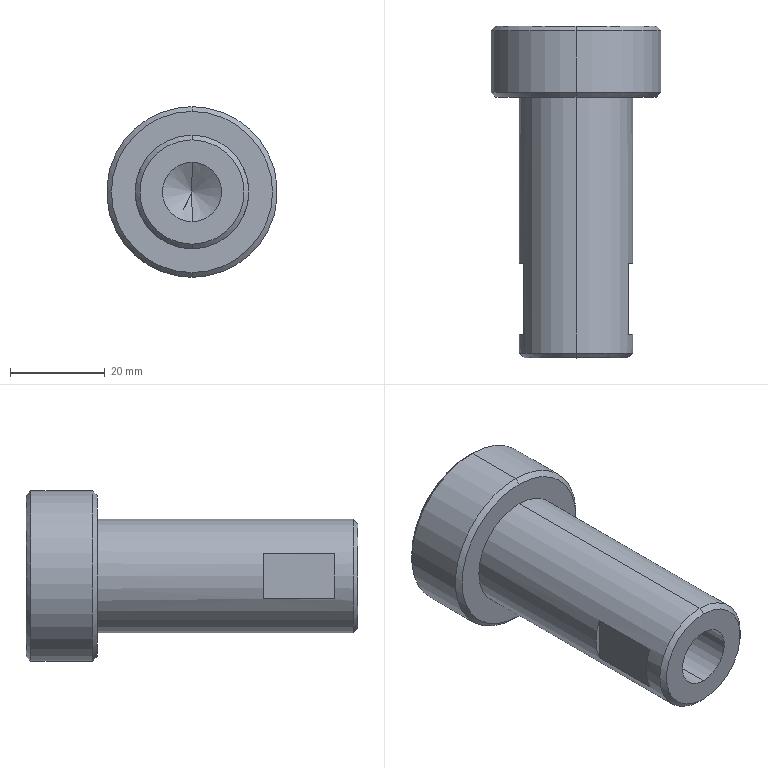Part | SolidWorks | features Chamfer 1, HoleWzd 1, ICE 1, Revolution 1 | 1 solid | 23 faces | box 36 x 70 x 36 mm | volume 37200 mm3 | plane 9 | cone 8 | cylinder 6 | commonest cylinder face diameters 12.5 x2 24 x2 36 x2
STEP:
#1=CARTESIAN_POINT('',(0.,-1.346,6.25));
#2=VERTEX_POINT('',#1);
#3=CARTESIAN_POINT('',(0.,-1.346,-6.25));
#4=VERTEX_POINT('',#3);
#5=CARTESIAN_POINT('',(0.,-1.346,0.));
#6=DIRECTION('',(0.,-1.,0.));
#7=DIRECTION('',(0.,0.,-1.));
#8=AXIS2_PLACEMENT_3D('',#5,#6,#7);
#9=CIRCLE('',#8,6.25);
#10=EDGE_CURVE('',#2,#4,#9,.T.);
#11=ORIENTED_EDGE('',*,*,#10,.F.);
#12=CARTESIAN_POINT('',(0.,-21.346,6.25));
#13=VERTEX_POINT('',#12);
#14=CARTESIAN_POINT('',(0.,-21.346,6.25));
#15=DIRECTION('',(0.,-1.,0.));
#16=VECTOR('',#15,1000.);
#17=LINE('',#14,#16);
#18=EDGE_CURVE('',#2,#13,#17,.T.);
#19=ORIENTED_EDGE('',*,*,#18,.T.);
#20=CARTESIAN_POINT('',(0.,-21.346,-6.25));
#21=VERTEX_POINT('',#20);
#22=CARTESIAN_POINT('',(0.,-21.346,0.));
#23=DIRECTION('',(0.,-1.,0.));
#24=DIRECTION('',(0.,0.,-1.));
#25=AXIS2_PLACEMENT_3D('',#22,#23,#24);
#26=CIRCLE('',#25,6.25);
#27=EDGE_CURVE('',#13,#21,#26,.T.);
#28=ORIENTED_EDGE('',*,*,#27,.T.);
#29=CARTESIAN_POINT('',(0.,-21.346,-6.25));
#30=DIRECTION('',(0.,-1.,0.));
#31=VECTOR('',#30,1000.);
#32=LINE('',#29,#31);
#33=EDGE_CURVE('',#4,#21,#32,.T.);
#34=ORIENTED_EDGE('',*,*,#33,.F.);
#35=EDGE_LOOP('',(#11,#19,#28,#34));
#36=FACE_OUTER_BOUND('',#35,.T.);
#37=CARTESIAN_POINT('',(0.,-21.346,0.));
#38=DIRECTION('',(0.,-1.,0.));
#39=DIRECTION('',(0.,0.,-1.));
#40=AXIS2_PLACEMENT_3D('',#37,#38,#39);
#41=CYLINDRICAL_SURFACE('',#40,6.25);
#42=ADVANCED_FACE('',(#36),#41,.F.);
#43=CARTESIAN_POINT('',(0.,2.409,0.));
#44=VERTEX_POINT('',#43);
#45=CARTESIAN_POINT('',(0.,-1.346,-6.25));
#46=DIRECTION('',(0.,-0.515,-0.8572));
#47=VECTOR('',#46,1000.);
#48=LINE('',#45,#47);
#49=EDGE_CURVE('',#44,#4,#48,.T.);
#50=ORIENTED_EDGE('',*,*,#49,.F.);
#51=CARTESIAN_POINT('',(0.,-1.346,6.25));
#52=DIRECTION('',(0.,-0.515,0.8572));
#53=VECTOR('',#52,1000.);
#54=LINE('',#51,#53);
#55=EDGE_CURVE('',#44,#2,#54,.T.);
#56=ORIENTED_EDGE('',*,*,#55,.T.);
#57=ORIENTED_EDGE('',*,*,#10,.T.);
#58=EDGE_LOOP('',(#50,#56,#57));
#59=FACE_OUTER_BOUND('',#58,.T.);
#60=CARTESIAN_POINT('',(0.,-1.346,0.));
#61=DIRECTION('',(0.,-1.,0.));
#62=DIRECTION('',(0.,0.,-1.));
#63=AXIS2_PLACEMENT_3D('',#60,#61,#62);
#64=CONICAL_SURFACE('',#63,6.25,1.03);
#65=ADVANCED_FACE('',(#59),#64,.F.);
#66=CARTESIAN_POINT('',(0.,48.654,17.));
#67=VERTEX_POINT('',#66);
#68=CARTESIAN_POINT('',(0.,48.654,-17.));
#69=VERTEX_POINT('',#68);
#70=CARTESIAN_POINT('',(0.,48.654,0.));
#71=DIRECTION('',(0.,1.,0.));
#72=DIRECTION('',(0.,0.,1.));
#73=AXIS2_PLACEMENT_3D('',#70,#71,#72);
#74=CIRCLE('',#73,17.);
#75=EDGE_CURVE('',#67,#69,#74,.T.);
#76=ORIENTED_EDGE('',*,*,#75,.F.);
#77=CARTESIAN_POINT('',(0.,47.654,18.));
#78=VERTEX_POINT('',#77);
#79=CARTESIAN_POINT('',(0.,48.654,17.));
#80=DIRECTION('',(0.,-0.7071,0.7071));
#81=VECTOR('',#80,1000.);
#82=LINE('',#79,#81);
#83=EDGE_CURVE('',#67,#78,#82,.T.);
#84=ORIENTED_EDGE('',*,*,#83,.T.);
#85=CARTESIAN_POINT('',(0.,47.654,-18.));
#86=VERTEX_POINT('',#85);
#87=CARTESIAN_POINT('',(0.,47.654,0.));
#88=DIRECTION('',(0.,-1.,0.));
#89=DIRECTION('',(0.,0.,1.));
#90=AXIS2_PLACEMENT_3D('',#87,#88,#89);
#91=CIRCLE('',#90,18.);
#92=EDGE_CURVE('',#86,#78,#91,.T.);
#93=ORIENTED_EDGE('',*,*,#92,.F.);
#94=CARTESIAN_POINT('',(0.,48.654,-17.));
#95=DIRECTION('',(0.,-0.7071,-0.7071));
#96=VECTOR('',#95,1000.);
#97=LINE('',#94,#96);
#98=EDGE_CURVE('',#69,#86,#97,.T.);
#99=ORIENTED_EDGE('',*,*,#98,.F.);
#100=EDGE_LOOP('',(#76,#84,#93,#99));
#101=FACE_OUTER_BOUND('',#100,.T.);
#102=CARTESIAN_POINT('',(0.,48.654,0.));
#103=DIRECTION('',(0.,-1.,0.));
#104=DIRECTION('',(0.,0.,-1.));
#105=AXIS2_PLACEMENT_3D('',#102,#103,#104);
#106=CONICAL_SURFACE('',#105,17.,0.7854);
#107=ADVANCED_FACE('',(#101),#106,.T.);
#108=CARTESIAN_POINT('',(0.,33.654,-17.));
#109=VERTEX_POINT('',#108);
#110=CARTESIAN_POINT('',(0.,33.654,17.));
#111=VERTEX_POINT('',#110);
#112=CARTESIAN_POINT('',(0.,33.654,0.));
#113=DIRECTION('',(0.,-1.,0.));
#114=DIRECTION('',(0.,0.,-1.));
#115=AXIS2_PLACEMENT_3D('',#112,#113,#114);
#116=CIRCLE('',#115,17.);
#117=EDGE_CURVE('',#109,#111,#116,.T.);
#118=ORIENTED_EDGE('',*,*,#117,.F.);
#119=CARTESIAN_POINT('',(0.,34.654,-18.));
#120=VERTEX_POINT('',#119);
#121=CARTESIAN_POINT('',(0.,34.654,-18.));
#122=DIRECTION('',(0.,0.7071,-0.7071));
#123=VECTOR('',#122,1000.);
#124=LINE('',#121,#123);
#125=EDGE_CURVE('',#109,#120,#124,.T.);
#126=ORIENTED_EDGE('',*,*,#125,.T.);
#127=CARTESIAN_POINT('',(0.,34.654,18.));
#128=VERTEX_POINT('',#127);
#129=CARTESIAN_POINT('',(0.,34.654,0.));
#130=DIRECTION('',(0.,1.,0.));
#131=DIRECTION('',(0.,0.,-1.));
#132=AXIS2_PLACEMENT_3D('',#129,#130,#131);
#133=CIRCLE('',#132,18.);
#134=EDGE_CURVE('',#128,#120,#133,.T.);
#135=ORIENTED_EDGE('',*,*,#134,.F.);
#136=CARTESIAN_POINT('',(0.,34.654,18.));
#137=DIRECTION('',(0.,0.7071,0.7071));
#138=VECTOR('',#137,1000.);
#139=LINE('',#136,#138);
#140=EDGE_CURVE('',#111,#128,#139,.T.);
#141=ORIENTED_EDGE('',*,*,#140,.F.);
#142=EDGE_LOOP('',(#118,#126,#135,#141));
#143=FACE_OUTER_BOUND('',#142,.T.);
#144=CARTESIAN_POINT('',(0.,34.654,0.));
#145=DIRECTION('',(0.,1.,0.));
#146=DIRECTION('',(0.,0.,1.));
#147=AXIS2_PLACEMENT_3D('',#144,#145,#146);
#148=CONICAL_SURFACE('',#147,18.,0.7854);
#149=ADVANCED_FACE('',(#143),#148,.T.);
#150=CARTESIAN_POINT('',(0.,-21.346,-11.));
#151=VERTEX_POINT('',#150);
#152=CARTESIAN_POINT('',(0.,-21.346,11.));
#153=VERTEX_POINT('',#152);
#154=CARTESIAN_POINT('',(0.,-21.346,0.));
#155=DIRECTION('',(0.,-1.,0.));
#156=DIRECTION('',(0.,0.,-1.));
#157=AXIS2_PLACEMENT_3D('',#154,#155,#156);
#158=CIRCLE('',#157,11.);
#159=EDGE_CURVE('',#151,#153,#158,.T.);
#160=ORIENTED_EDGE('',*,*,#159,.F.);
#161=CARTESIAN_POINT('',(0.,-20.346,-12.));
#162=VERTEX_POINT('',#161);
#163=CARTESIAN_POINT('',(0.,-20.346,-12.));
#164=DIRECTION('',(0.,0.7071,-0.7071));
#165=VECTOR('',#164,1000.);
#166=LINE('',#163,#165);
#167=EDGE_CURVE('',#151,#162,#166,.T.);
#168=ORIENTED_EDGE('',*,*,#167,.T.);
#169=CARTESIAN_POINT('',(0.,-20.346,12.));
#170=VERTEX_POINT('',#169);
#171=CARTESIAN_POINT('',(0.,-20.346,0.));
#172=DIRECTION('',(0.,1.,0.));
#173=DIRECTION('',(0.,0.,-1.));
#174=AXIS2_PLACEMENT_3D('',#171,#172,#173);
#175=CIRCLE('',#174,12.);
#176=EDGE_CURVE('',#170,#162,#175,.T.);
#177=ORIENTED_EDGE('',*,*,#176,.F.);
#178=CARTESIAN_POINT('',(0.,-20.346,12.));
#179=DIRECTION('',(0.,0.7071,0.7071));
#180=VECTOR('',#179,1000.);
#181=LINE('',#178,#180);
#182=EDGE_CURVE('',#153,#170,#181,.T.);
#183=ORIENTED_EDGE('',*,*,#182,.F.);
#184=EDGE_LOOP('',(#160,#168,#177,#183));
#185=FACE_OUTER_BOUND('',#184,.T.);
#186=CARTESIAN_POINT('',(0.,-20.346,0.));
#187=DIRECTION('',(0.,1.,0.));
#188=DIRECTION('',(0.,0.,1.));
#189=AXIS2_PLACEMENT_3D('',#186,#187,#188);
#190=CONICAL_SURFACE('',#189,12.,0.7854);
#191=ADVANCED_FACE('',(#185),#190,.T.);
#192=CARTESIAN_POINT('',(11.,-1.346,4.796));
#193=VERTEX_POINT('',#192);
#194=CARTESIAN_POINT('',(11.,-16.346,4.796));
#195=VERTEX_POINT('',#194);
#196=CARTESIAN_POINT('',(11.,14.106,4.796));
#197=DIRECTION('',(0.,-1.,0.));
#198=VECTOR('',#197,1000.);
#199=LINE('',#196,#198);
#200=EDGE_CURVE('',#193,#195,#199,.T.);
#201=ORIENTED_EDGE('',*,*,#200,.F.);
#202=CARTESIAN_POINT('',(11.,-1.346,-4.796));
#203=VERTEX_POINT('',#202);
#204=CARTESIAN_POINT('',(0.,-1.346,0.));
#205=DIRECTION('',(0.,-1.,0.));
#206=DIRECTION('',(0.,0.,1.));
#207=AXIS2_PLACEMENT_3D('',#204,#205,#206);
#208=CIRCLE('',#207,12.);
#209=EDGE_CURVE('',#203,#193,#208,.T.);
#210=ORIENTED_EDGE('',*,*,#209,.F.);
#211=CARTESIAN_POINT('',(11.,-16.346,-4.796));
#212=VERTEX_POINT('',#211);
#213=CARTESIAN_POINT('',(11.,14.106,-4.796));
#214=DIRECTION('',(0.,1.,0.));
#215=VECTOR('',#214,1000.);
#216=LINE('',#213,#215);
#217=EDGE_CURVE('',#212,#203,#216,.T.);
#218=ORIENTED_EDGE('',*,*,#217,.F.);
#219=CARTESIAN_POINT('',(0.,-16.346,0.));
#220=DIRECTION('',(0.,1.,0.));
#221=DIRECTION('',(0.,0.,-1.));
#222=AXIS2_PLACEMENT_3D('',#219,#220,#221);
#223=CIRCLE('',#222,12.);
#224=EDGE_CURVE('',#195,#212,#223,.T.);
#225=ORIENTED_EDGE('',*,*,#224,.F.);
#226=EDGE_LOOP('',(#201,#210,#218,#225));
#227=FACE_BOUND('',#226,.T.);
#228=ORIENTED_EDGE('',*,*,#176,.T.);
#229=CARTESIAN_POINT('',(0.,33.654,-12.));
#230=VERTEX_POINT('',#229);
#231=CARTESIAN_POINT('',(0.,14.106,-12.));
#232=DIRECTION('',(0.,1.,0.));
#233=VECTOR('',#232,1000.);
#234=LINE('',#231,#233);
#235=EDGE_CURVE('',#162,#230,#234,.T.);
#236=ORIENTED_EDGE('',*,*,#235,.T.);
#237=CARTESIAN_POINT('',(0.,33.654,12.));
#238=VERTEX_POINT('',#237);
#239=CARTESIAN_POINT('',(0.,33.654,0.));
#240=DIRECTION('',(0.,1.,0.));
#241=DIRECTION('',(0.,0.,1.));
#242=AXIS2_PLACEMENT_3D('',#239,#240,#241);
#243=CIRCLE('',#242,12.);
#244=EDGE_CURVE('',#238,#230,#243,.T.);
#245=ORIENTED_EDGE('',*,*,#244,.F.);
#246=CARTESIAN_POINT('',(0.,14.106,12.));
#247=DIRECTION('',(0.,1.,0.));
#248=VECTOR('',#247,1000.);
#249=LINE('',#246,#248);
#250=EDGE_CURVE('',#170,#238,#249,.T.);
#251=ORIENTED_EDGE('',*,*,#250,.F.);
#252=EDGE_LOOP('',(#228,#236,#245,#251));
#253=FACE_OUTER_BOUND('',#252,.T.);
#254=CARTESIAN_POINT('',(0.,14.106,0.));
#255=DIRECTION('',(0.,1.,0.));
#256=DIRECTION('',(0.,0.,1.));
#257=AXIS2_PLACEMENT_3D('',#254,#255,#256);
#258=CYLINDRICAL_SURFACE('',#257,12.);
#259=ADVANCED_FACE('',(#227,#253),#258,.T.);
#260=ORIENTED_EDGE('',*,*,#134,.T.);
#261=CARTESIAN_POINT('',(0.,14.106,-18.));
#262=DIRECTION('',(0.,1.,0.));
#263=VECTOR('',#262,1000.);
#264=LINE('',#261,#263);
#265=EDGE_CURVE('',#120,#86,#264,.T.);
#266=ORIENTED_EDGE('',*,*,#265,.T.);
#267=ORIENTED_EDGE('',*,*,#92,.T.);
#268=CARTESIAN_POINT('',(0.,14.106,18.));
#269=DIRECTION('',(0.,1.,0.));
#270=VECTOR('',#269,1000.);
#271=LINE('',#268,#270);
#272=EDGE_CURVE('',#128,#78,#271,.T.);
#273=ORIENTED_EDGE('',*,*,#272,.F.);
#274=EDGE_LOOP('',(#260,#266,#267,#273));
#275=FACE_OUTER_BOUND('',#274,.T.);
#276=CARTESIAN_POINT('',(0.,14.106,0.));
#277=DIRECTION('',(0.,1.,0.));
#278=DIRECTION('',(0.,0.,1.));
#279=AXIS2_PLACEMENT_3D('',#276,#277,#278);
#280=CYLINDRICAL_SURFACE('',#279,18.);
#281=ADVANCED_FACE('',(#275),#280,.T.);
#282=CARTESIAN_POINT('',(0.,48.654,0.));
#283=DIRECTION('',(0.,1.,0.));
#284=DIRECTION('',(0.,0.,1.));
#285=AXIS2_PLACEMENT_3D('',#282,#283,#284);
#286=CIRCLE('',#285,17.);
#287=EDGE_CURVE('',#69,#67,#286,.T.);
#288=ORIENTED_EDGE('',*,*,#287,.T.);
#289=ORIENTED_EDGE('',*,*,#75,.T.);
#290=EDGE_LOOP('',(#288,#289));
#291=FACE_OUTER_BOUND('',#290,.T.);
#292=CARTESIAN_POINT('',(0.,48.654,0.));
#293=DIRECTION('',(0.,1.,0.));
#294=DIRECTION('',(0.,0.,1.));
#295=AXIS2_PLACEMENT_3D('',#292,#293,#294);
#296=PLANE('',#295);
#297=ADVANCED_FACE('',(#291),#296,.T.);
#298=ORIENTED_EDGE('',*,*,#265,.F.);
#299=CARTESIAN_POINT('',(0.,34.654,0.));
#300=DIRECTION('',(0.,1.,0.));
#301=DIRECTION('',(0.,0.,-1.));
#302=AXIS2_PLACEMENT_3D('',#299,#300,#301);
#303=CIRCLE('',#302,18.);
#304=EDGE_CURVE('',#120,#128,#303,.T.);
#305=ORIENTED_EDGE('',*,*,#304,.T.);
#306=ORIENTED_EDGE('',*,*,#272,.T.);
#307=CARTESIAN_POINT('',(0.,47.654,0.));
#308=DIRECTION('',(0.,-1.,0.));
#309=DIRECTION('',(0.,0.,1.));
#310=AXIS2_PLACEMENT_3D('',#307,#308,#309);
#311=CIRCLE('',#310,18.);
#312=EDGE_CURVE('',#78,#86,#311,.T.);
#313=ORIENTED_EDGE('',*,*,#312,.T.);
#314=EDGE_LOOP('',(#298,#305,#306,#313));
#315=FACE_OUTER_BOUND('',#314,.T.);
#316=CARTESIAN_POINT('',(0.,14.106,0.));
#317=DIRECTION('',(0.,1.,0.));
#318=DIRECTION('',(0.,0.,1.));
#319=AXIS2_PLACEMENT_3D('',#316,#317,#318);
#320=CYLINDRICAL_SURFACE('',#319,18.);
#321=ADVANCED_FACE('',(#315),#320,.T.);
#322=CARTESIAN_POINT('',(0.,33.654,0.));
#323=DIRECTION('',(0.,-1.,0.));
#324=DIRECTION('',(0.,0.,-1.));
#325=AXIS2_PLACEMENT_3D('',#322,#323,#324);
#326=CIRCLE('',#325,17.);
#327=EDGE_CURVE('',#111,#109,#326,.T.);
#328=ORIENTED_EDGE('',*,*,#327,.T.);
#329=ORIENTED_EDGE('',*,*,#117,.T.);
#330=EDGE_LOOP('',(#328,#329));
#331=FACE_OUTER_BOUND('',#330,.T.);
#332=ORIENTED_EDGE('',*,*,#244,.T.);
#333=CARTESIAN_POINT('',(0.,33.654,0.));
#334=DIRECTION('',(0.,1.,0.));
#335=DIRECTION('',(0.,0.,1.));
#336=AXIS2_PLACEMENT_3D('',#333,#334,#335);
#337=CIRCLE('',#336,12.);
#338=EDGE_CURVE('',#230,#238,#337,.T.);
#339=ORIENTED_EDGE('',*,*,#338,.T.);
#340=EDGE_LOOP('',(#332,#339));
#341=FACE_BOUND('',#340,.T.);
#342=CARTESIAN_POINT('',(-18.,33.654,0.));
#343=DIRECTION('',(0.,-1.,0.));
#344=DIRECTION('',(0.,0.,-1.));
#345=AXIS2_PLACEMENT_3D('',#342,#343,#344);
#346=PLANE('',#345);
#347=ADVANCED_FACE('',(#331,#341),#346,.T.);
#348=ORIENTED_EDGE('',*,*,#235,.F.);
#349=CARTESIAN_POINT('',(0.,-20.346,0.));
#350=DIRECTION('',(0.,1.,0.));
#351=DIRECTION('',(0.,0.,-1.));
#352=AXIS2_PLACEMENT_3D('',#349,#350,#351);
#353=CIRCLE('',#352,12.);
#354=EDGE_CURVE('',#162,#170,#353,.T.);
#355=ORIENTED_EDGE('',*,*,#354,.T.);
#356=ORIENTED_EDGE('',*,*,#250,.T.);
#357=ORIENTED_EDGE('',*,*,#338,.F.);
#358=EDGE_LOOP('',(#348,#355,#356,#357));
#359=FACE_OUTER_BOUND('',#358,.T.);
#360=CARTESIAN_POINT('',(-11.,-1.346,4.796));
#361=VERTEX_POINT('',#360);
#362=CARTESIAN_POINT('',(-11.,-1.346,-4.796));
#363=VERTEX_POINT('',#362);
#364=CARTESIAN_POINT('',(0.,-1.346,0.));
#365=DIRECTION('',(0.,-1.,0.));
#366=DIRECTION('',(0.,0.,1.));
#367=AXIS2_PLACEMENT_3D('',#364,#365,#366);
#368=CIRCLE('',#367,12.);
#369=EDGE_CURVE('',#361,#363,#368,.T.);
#370=ORIENTED_EDGE('',*,*,#369,.F.);
#371=CARTESIAN_POINT('',(-11.,-16.346,4.796));
#372=VERTEX_POINT('',#371);
#373=CARTESIAN_POINT('',(-11.,14.106,4.796));
#374=DIRECTION('',(0.,1.,0.));
#375=VECTOR('',#374,1000.);
#376=LINE('',#373,#375);
#377=EDGE_CURVE('',#372,#361,#376,.T.);
#378=ORIENTED_EDGE('',*,*,#377,.F.);
#379=CARTESIAN_POINT('',(-11.,-16.346,-4.796));
#380=VERTEX_POINT('',#379);
#381=CARTESIAN_POINT('',(0.,-16.346,0.));
#382=DIRECTION('',(0.,1.,0.));
#383=DIRECTION('',(0.,0.,-1.));
#384=AXIS2_PLACEMENT_3D('',#381,#382,#383);
#385=CIRCLE('',#384,12.);
#386=EDGE_CURVE('',#380,#372,#385,.T.);
#387=ORIENTED_EDGE('',*,*,#386,.F.);
#388=CARTESIAN_POINT('',(-11.,14.106,-4.796));
#389=DIRECTION('',(0.,-1.,0.));
#390=VECTOR('',#389,1000.);
#391=LINE('',#388,#390);
#392=EDGE_CURVE('',#363,#380,#391,.T.);
#393=ORIENTED_EDGE('',*,*,#392,.F.);
#394=EDGE_LOOP('',(#370,#378,#387,#393));
#395=FACE_BOUND('',#394,.T.);
#396=CARTESIAN_POINT('',(0.,14.106,0.));
#397=DIRECTION('',(0.,1.,0.));
#398=DIRECTION('',(0.,0.,1.));
#399=AXIS2_PLACEMENT_3D('',#396,#397,#398);
#400=CYLINDRICAL_SURFACE('',#399,12.);
#401=ADVANCED_FACE('',(#359,#395),#400,.T.);
#402=CARTESIAN_POINT('',(0.,-21.346,0.));
#403=DIRECTION('',(0.,-1.,0.));
#404=DIRECTION('',(0.,0.,-1.));
#405=AXIS2_PLACEMENT_3D('',#402,#403,#404);
#406=CIRCLE('',#405,6.25);
#407=EDGE_CURVE('',#21,#13,#406,.T.);
#408=ORIENTED_EDGE('',*,*,#407,.F.);
#409=ORIENTED_EDGE('',*,*,#27,.F.);
#410=EDGE_LOOP('',(#408,#409));
#411=FACE_BOUND('',#410,.T.);
#412=CARTESIAN_POINT('',(0.,-21.346,0.));
#413=DIRECTION('',(0.,-1.,0.));
#414=DIRECTION('',(0.,0.,-1.));
#415=AXIS2_PLACEMENT_3D('',#412,#413,#414);
#416=CIRCLE('',#415,11.);
#417=EDGE_CURVE('',#153,#151,#416,.T.);
#418=ORIENTED_EDGE('',*,*,#417,.T.);
#419=ORIENTED_EDGE('',*,*,#159,.T.);
#420=EDGE_LOOP('',(#418,#419));
#421=FACE_OUTER_BOUND('',#420,.T.);
#422=CARTESIAN_POINT('',(-12.,-21.346,0.));
#423=DIRECTION('',(0.,-1.,0.));
#424=DIRECTION('',(0.,0.,-1.));
#425=AXIS2_PLACEMENT_3D('',#422,#423,#424);
#426=PLANE('',#425);
#427=ADVANCED_FACE('',(#411,#421),#426,.T.);
#428=ORIENTED_EDGE('',*,*,#167,.F.);
#429=ORIENTED_EDGE('',*,*,#417,.F.);
#430=ORIENTED_EDGE('',*,*,#182,.T.);
#431=ORIENTED_EDGE('',*,*,#354,.F.);
#432=EDGE_LOOP('',(#428,#429,#430,#431));
#433=FACE_OUTER_BOUND('',#432,.T.);
#434=CARTESIAN_POINT('',(0.,-20.346,0.));
#435=DIRECTION('',(0.,1.,0.));
#436=DIRECTION('',(0.,0.,1.));
#437=AXIS2_PLACEMENT_3D('',#434,#435,#436);
#438=CONICAL_SURFACE('',#437,12.,0.7854);
#439=ADVANCED_FACE('',(#433),#438,.T.);
#440=ORIENTED_EDGE('',*,*,#125,.F.);
#441=ORIENTED_EDGE('',*,*,#327,.F.);
#442=ORIENTED_EDGE('',*,*,#140,.T.);
#443=ORIENTED_EDGE('',*,*,#304,.F.);
#444=EDGE_LOOP('',(#440,#441,#442,#443));
#445=FACE_OUTER_BOUND('',#444,.T.);
#446=CARTESIAN_POINT('',(0.,34.654,0.));
#447=DIRECTION('',(0.,1.,0.));
#448=DIRECTION('',(0.,0.,1.));
#449=AXIS2_PLACEMENT_3D('',#446,#447,#448);
#450=CONICAL_SURFACE('',#449,18.,0.7854);
#451=ADVANCED_FACE('',(#445),#450,.T.);
#452=ORIENTED_EDGE('',*,*,#83,.F.);
#453=ORIENTED_EDGE('',*,*,#287,.F.);
#454=ORIENTED_EDGE('',*,*,#98,.T.);
#455=ORIENTED_EDGE('',*,*,#312,.F.);
#456=EDGE_LOOP('',(#452,#453,#454,#455));
#457=FACE_OUTER_BOUND('',#456,.T.);
#458=CARTESIAN_POINT('',(0.,48.654,0.));
#459=DIRECTION('',(0.,-1.,0.));
#460=DIRECTION('',(0.,0.,-1.));
#461=AXIS2_PLACEMENT_3D('',#458,#459,#460);
#462=CONICAL_SURFACE('',#461,17.,0.7854);
#463=ADVANCED_FACE('',(#457),#462,.T.);
#464=ORIENTED_EDGE('',*,*,#209,.T.);
#465=CARTESIAN_POINT('',(11.,-1.346,-18.));
#466=DIRECTION('',(0.,0.,1.));
#467=VECTOR('',#466,1000.);
#468=LINE('',#465,#467);
#469=EDGE_CURVE('',#203,#193,#468,.T.);
#470=ORIENTED_EDGE('',*,*,#469,.F.);
#471=EDGE_LOOP('',(#464,#470));
#472=FACE_OUTER_BOUND('',#471,.T.);
#473=CARTESIAN_POINT('',(12.,-1.346,-18.));
#474=DIRECTION('',(0.,1.,0.));
#475=DIRECTION('',(0.,0.,1.));
#476=AXIS2_PLACEMENT_3D('',#473,#474,#475);
#477=PLANE('',#476);
#478=ADVANCED_FACE('',(#472),#477,.F.);
#479=CARTESIAN_POINT('',(11.,-16.346,-18.));
#480=DIRECTION('',(0.,0.,1.));
#481=VECTOR('',#480,1000.);
#482=LINE('',#479,#481);
#483=EDGE_CURVE('',#212,#195,#482,.T.);
#484=ORIENTED_EDGE('',*,*,#483,.T.);
#485=ORIENTED_EDGE('',*,*,#224,.T.);
#486=EDGE_LOOP('',(#484,#485));
#487=FACE_OUTER_BOUND('',#486,.T.);
#488=CARTESIAN_POINT('',(12.,-16.346,-18.));
#489=DIRECTION('',(0.,-1.,0.));
#490=DIRECTION('',(0.,0.,-1.));
#491=AXIS2_PLACEMENT_3D('',#488,#489,#490);
#492=PLANE('',#491);
#493=ADVANCED_FACE('',(#487),#492,.F.);
#494=ORIENTED_EDGE('',*,*,#200,.T.);
#495=ORIENTED_EDGE('',*,*,#483,.F.);
#496=ORIENTED_EDGE('',*,*,#217,.T.);
#497=ORIENTED_EDGE('',*,*,#469,.T.);
#498=EDGE_LOOP('',(#494,#495,#496,#497));
#499=FACE_OUTER_BOUND('',#498,.T.);
#500=CARTESIAN_POINT('',(11.,-1.346,-18.));
#501=DIRECTION('',(-1.,0.,0.));
#502=DIRECTION('',(0.,-1.,0.));
#503=AXIS2_PLACEMENT_3D('',#500,#501,#502);
#504=PLANE('',#503);
#505=ADVANCED_FACE('',(#499),#504,.F.);
#506=CARTESIAN_POINT('',(-11.,-1.346,-18.));
#507=DIRECTION('',(0.,0.,1.));
#508=VECTOR('',#507,1000.);
#509=LINE('',#506,#508);
#510=EDGE_CURVE('',#363,#361,#509,.T.);
#511=ORIENTED_EDGE('',*,*,#510,.T.);
#512=ORIENTED_EDGE('',*,*,#369,.T.);
#513=EDGE_LOOP('',(#511,#512));
#514=FACE_OUTER_BOUND('',#513,.T.);
#515=CARTESIAN_POINT('',(-12.,-1.346,-18.));
#516=DIRECTION('',(0.,1.,0.));
#517=DIRECTION('',(0.,0.,1.));
#518=AXIS2_PLACEMENT_3D('',#515,#516,#517);
#519=PLANE('',#518);
#520=ADVANCED_FACE('',(#514),#519,.F.);
#521=ORIENTED_EDGE('',*,*,#392,.T.);
#522=CARTESIAN_POINT('',(-11.,-16.346,-18.));
#523=DIRECTION('',(0.,0.,1.));
#524=VECTOR('',#523,1000.);
#525=LINE('',#522,#524);
#526=EDGE_CURVE('',#380,#372,#525,.T.);
#527=ORIENTED_EDGE('',*,*,#526,.T.);
#528=ORIENTED_EDGE('',*,*,#377,.T.);
#529=ORIENTED_EDGE('',*,*,#510,.F.);
#530=EDGE_LOOP('',(#521,#527,#528,#529));
#531=FACE_OUTER_BOUND('',#530,.T.);
#532=CARTESIAN_POINT('',(-11.,-1.346,-18.));
#533=DIRECTION('',(1.,0.,0.));
#534=DIRECTION('',(0.,1.,0.));
#535=AXIS2_PLACEMENT_3D('',#532,#533,#534);
#536=PLANE('',#535);
#537=ADVANCED_FACE('',(#531),#536,.F.);
#538=ORIENTED_EDGE('',*,*,#526,.F.);
#539=ORIENTED_EDGE('',*,*,#386,.T.);
#540=EDGE_LOOP('',(#538,#539));
#541=FACE_OUTER_BOUND('',#540,.T.);
#542=CARTESIAN_POINT('',(-12.,-16.346,-18.));
#543=DIRECTION('',(0.,-1.,0.));
#544=DIRECTION('',(0.,0.,-1.));
#545=AXIS2_PLACEMENT_3D('',#542,#543,#544);
#546=PLANE('',#545);
#547=ADVANCED_FACE('',(#541),#546,.F.);
#548=ORIENTED_EDGE('',*,*,#55,.F.);
#549=ORIENTED_EDGE('',*,*,#49,.T.);
#550=CARTESIAN_POINT('',(0.,-1.346,0.));
#551=DIRECTION('',(0.,-1.,0.));
#552=DIRECTION('',(0.,0.,-1.));
#553=AXIS2_PLACEMENT_3D('',#550,#551,#552);
#554=CIRCLE('',#553,6.25);
#555=EDGE_CURVE('',#4,#2,#554,.T.);
#556=ORIENTED_EDGE('',*,*,#555,.T.);
#557=EDGE_LOOP('',(#548,#549,#556));
#558=FACE_OUTER_BOUND('',#557,.T.);
#559=CARTESIAN_POINT('',(0.,-1.346,0.));
#560=DIRECTION('',(0.,-1.,0.));
#561=DIRECTION('',(0.,0.,-1.));
#562=AXIS2_PLACEMENT_3D('',#559,#560,#561);
#563=CONICAL_SURFACE('',#562,6.25,1.03);
#564=ADVANCED_FACE('',(#558),#563,.F.);
#565=ORIENTED_EDGE('',*,*,#18,.F.);
#566=ORIENTED_EDGE('',*,*,#555,.F.);
#567=ORIENTED_EDGE('',*,*,#33,.T.);
#568=ORIENTED_EDGE('',*,*,#407,.T.);
#569=EDGE_LOOP('',(#565,#566,#567,#568));
#570=FACE_OUTER_BOUND('',#569,.T.);
#571=CARTESIAN_POINT('',(0.,-21.346,0.));
#572=DIRECTION('',(0.,-1.,0.));
#573=DIRECTION('',(0.,0.,-1.));
#574=AXIS2_PLACEMENT_3D('',#571,#572,#573);
#575=CYLINDRICAL_SURFACE('',#574,6.25);
#576=ADVANCED_FACE('',(#570),#575,.F.);
#577=CLOSED_SHELL('',(#42,#65,#107,#149,#191,#259,#281,#297,#321,#347,#401,#427,#439,#451,#463,#478,#493,#505,#520,#537,#547,#564,#576));
#578=MANIFOLD_SOLID_BREP('',#577);
#579=CARTESIAN_POINT('',(0.,0.,0.));
#580=DIRECTION('',(0.,0.,1.));
#581=DIRECTION('',(1.,0.,0.));
#582=AXIS2_PLACEMENT_3D('',#579,#580,#581);
#583=(LENGTH_UNIT()NAMED_UNIT(*)SI_UNIT(.MILLI.,.METRE.));
#584=UNCERTAINTY_MEASURE_WITH_UNIT(LENGTH_MEASURE(0.00001),#583,'','');
#585=(NAMED_UNIT(*)PLANE_ANGLE_UNIT()SI_UNIT($,.RADIAN.));
#586=(NAMED_UNIT(*)SI_UNIT($,.STERADIAN.)SOLID_ANGLE_UNIT());
#587=(GEOMETRIC_REPRESENTATION_CONTEXT(3)GLOBAL_UNCERTAINTY_ASSIGNED_CONTEXT((#584))GLOBAL_UNIT_ASSIGNED_CONTEXT((#583,#585,#586))REPRESENTATION_CONTEXT('',''));
#588=ADVANCED_BREP_SHAPE_REPRESENTATION('',(#578,#582),#587);